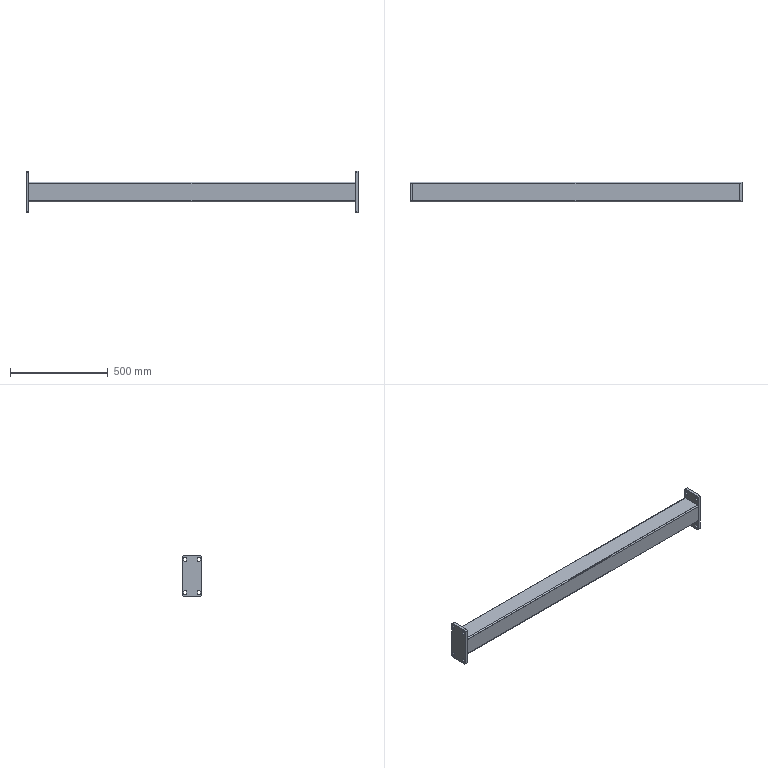Part | SolidWorks | features HoleWzd 1, ICE 1, MirrorSolid 1, WeldMemberFeat 1, WeldmentFeature 1 | 3 solids | 78 faces | box 1695 x 100 x 210 mm | volume 2614218 mm3 | plane 46 | cylinder 32 | commonest cylinder face diameters 13.5 x24 6.4 x4 12.8 x4